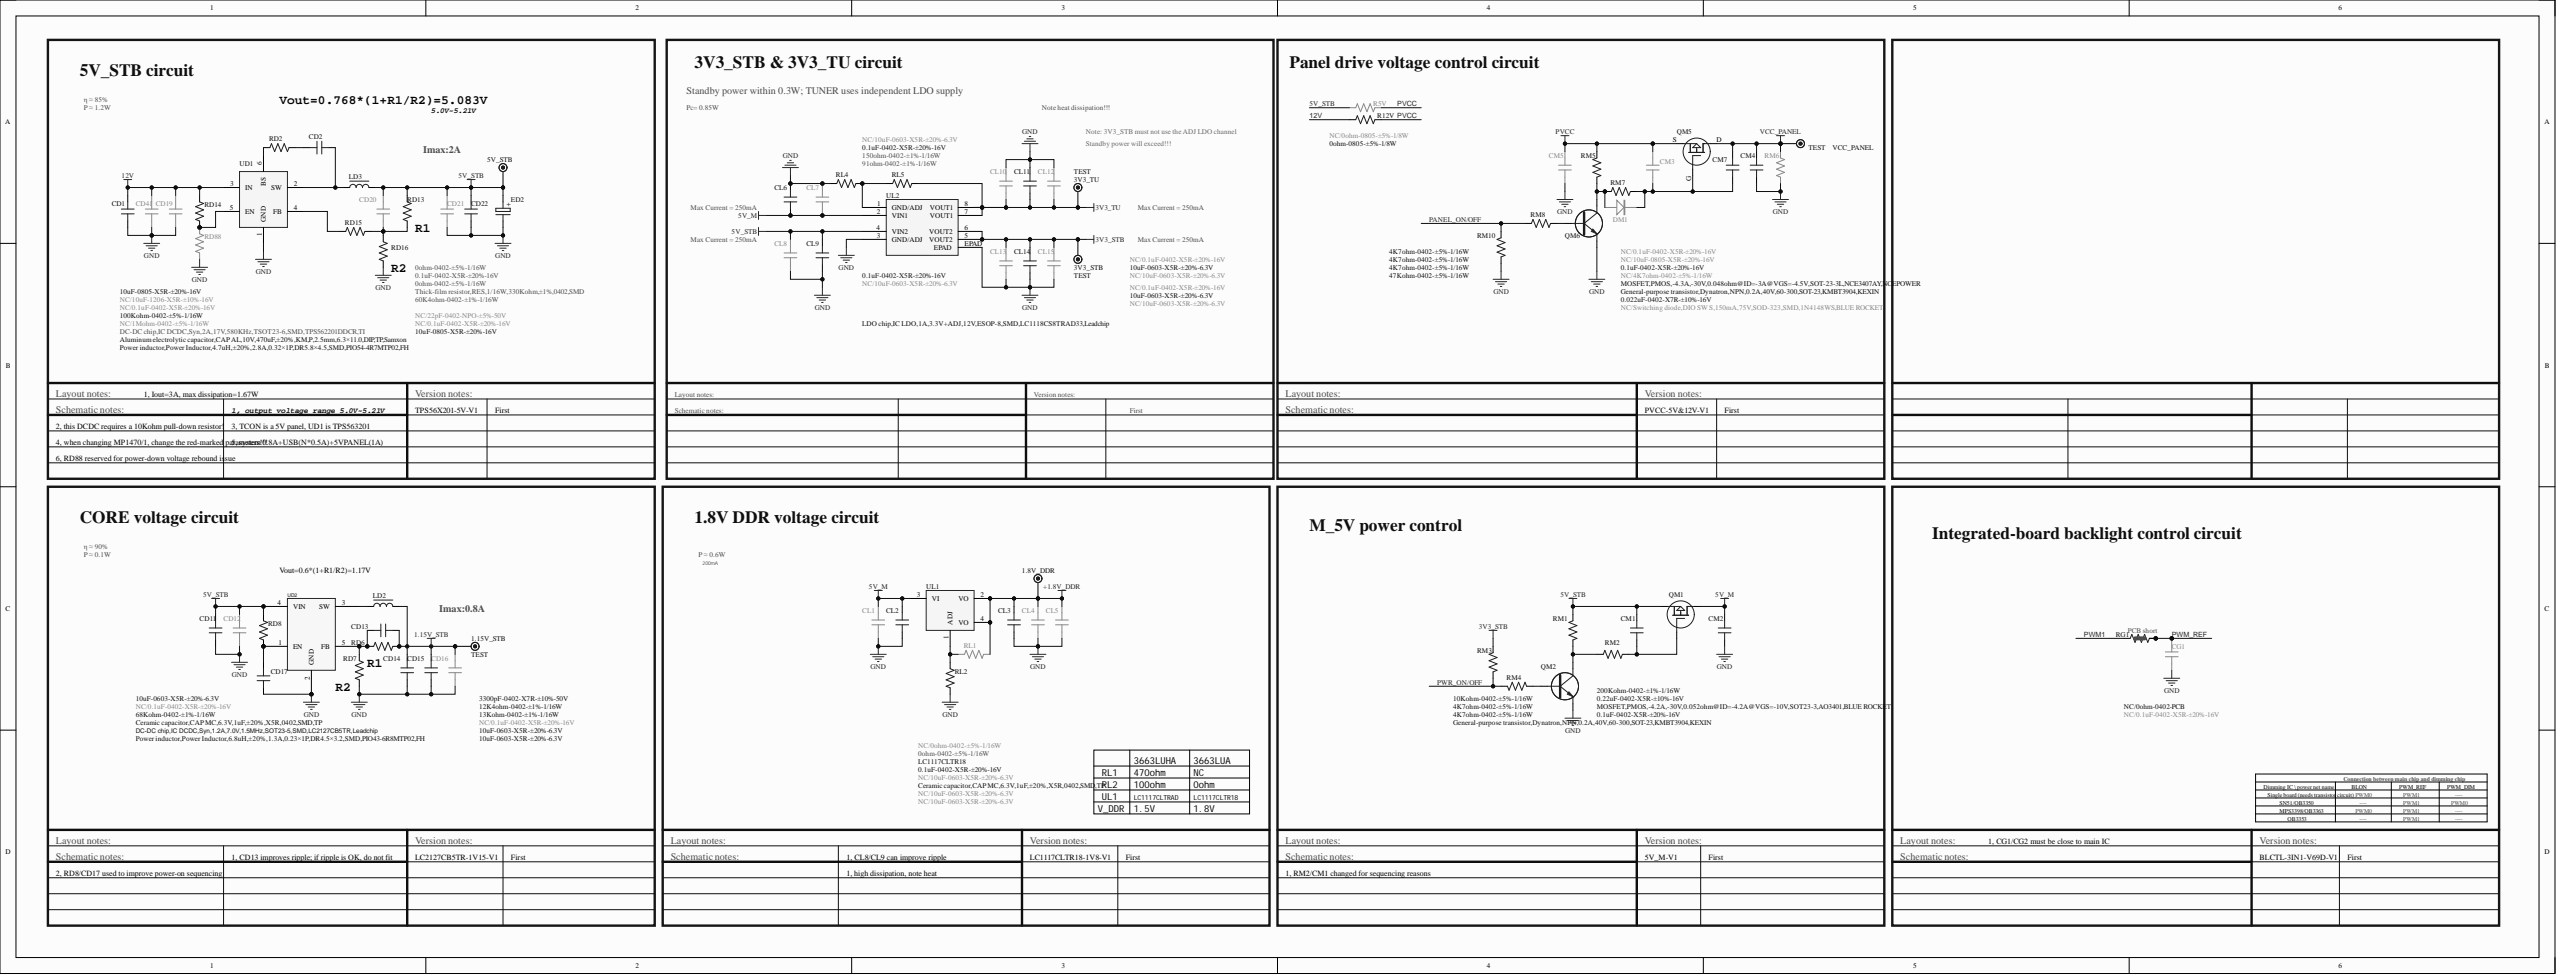Circuit board | Altium Designer | 574 parts | 274 nets | one sheet of the schematic
Parts on this sheet (reference | value | footprint):
1.8V_DDR | TEST | TP
1.15V_STB | TEST | TP
3V3_TU | TEST | TP
CD1 | 10uF-0805-X5R-±20%-16V | C0805
CD2 | 0.1uF-0402-X5R-±20%-16V | C0402
CD11 | 10uF-0603-X5R-±20%-6.3V | C0603
CD12 | NC/0.1uF-0402-X5R-±20%-16V | C0402
CD13 | 3300pF-0402-X7R-±10%-50V | C0402
CD14 | 10uF-0603-X5R-±20%-6.3V | C0603
CD15 | 10uF-0603-X5R-±20%-6.3V | C0603
CD16 | NC/0.1uF-0402-X5R-±20%-16V | C0402
CD17 | Ceramic capacitor,CAP MC,6.3V,1uF,±20%,X5R,0402,SMD,TP | C0402
CD19 | NC/0.1uF-0402-X5R-±20%-16V | C0402
CD20 | NC/22pF-0402-NPO-±5%-50V | C0402
CD21 | NC/0.1uF-0402-X5R-±20%-16V | C0402
CD22 | 10uF-0805-X5R-±20%-16V | C0805
CD41 | NC/10uF-1206-X5R-±10%-16V | C1206
CG1 | NC/0.1uF-0402-X5R-±20%-16V | C0402
CL1 | NC/10uF-0603-X5R-±20%-6.3V | C0603
CL2 | 0.1uF-0402-X5R-±20%-16V | C0402
CL3 | Ceramic capacitor,CAP MC,6.3V,1uF,±20%,X5R,0402,SMD,TP | C0402
CL4 | NC/10uF-0603-X5R-±20%-6.3V | C0603
CL5 | NC/10uF-0603-X5R-±20%-6.3V | C0603
CL6 | 0.1uF-0402-X5R-±20%-16V | C0402
CL7 | NC/10uF-0603-X5R-±20%-6.3V | C0603
CL8 | NC/10uF-0603-X5R-±20%-6.3V | C0603
CL9 | 0.1uF-0402-X5R-±20%-16V | C0402
CL10 | NC/0.1uF-0402-X5R-±20%-16V | C0402
CL11 | 10uF-0603-X5R-±20%-6.3V | C0603
CL12 | NC/10uF-0603-X5R-±20%-6.3V | C0603
CL13 | NC/0.1uF-0402-X5R-±20%-16V | C0402
CL14 | 10uF-0603-X5R-±20%-6.3V | C0603
CL15 | NC/10uF-0603-X5R-±20%-6.3V | C0603
CM1 | 0.22uF-0402-X5R-±10%-16V | C0402
CM2 | 0.1uF-0402-X5R-±20%-16V | C0402
CM3 | NC/0.1uF-0402-X5R-±20%-16V | C0402
CM4 | 0.1uF-0402-X5R-±20%-16V | C0402
CM5 | NC/10uF-0805-X5R-±20%-16V | C0805
CM7 | 0.022uF-0402-X7R-±10%-16V | C0402
DM1 | NC/Switching diode,DIO SW S,150mA,75V,SOD-323,SMD,1N4148WS,BLUE ROCKET | DIODE-S-12
ED2 | Aluminum electrolytic capacitor,CAP AL,10V,470uF,±20%,KM,P,2.5mm,6.3×11.0,DIP,TP,Samxon | EC(6.3*11)-V-2.5
LD2 | Power inductor,Power Inductor,6.8uH,±20%,1.3A,0.23×1P,DR4.5×3.2,SMD,PIO43-6R8MTP02,FH | L(4.5*3.5)-S
LD3 | Power inductor,Power Inductor,4.7uH,±20%,2.8A,0.32×1P,DR5.8×4.5,SMD,PIO54-4R7MTP02,FH | L(6.0*4.5)-S
QM1 | MOSFET,PMOS,-4.2A,-30V,0.052ohm@ID=-4.2A@VGS=-10V,SOT23-3,AO3401,BLUE ROCKET | SOT-23-1
QM2 | General-purpose transistor,Dynatron,NPN,0.2A,40V,60-300,SOT-23,KMBT3904,KEXIN | SOT-23
QM5 | MOSFET,PMOS,-4.3A,-30V,0.048ohm@ID=-3A@VGS=-4.5V,SOT-23-3L,NCE3407AY,NCEPOWER | SOT-23-1
QM6 | General-purpose transistor,Dynatron,NPN,0.2A,40V,60-300,SOT-23,KMBT3904,KEXIN | SOT-23
R5V | NC/0ohm-0805-±5%-1/8W | R0805
R12V | 0ohm-0805-±5%-1/8W | R0805
RD2 | 0ohm-0402-±5%-1/16W | R0402
RD6 | 12K4ohm-0402-±1%-1/16W | R0402
RD7 | 13Kohm-0402-±1%-1/16W | R0402
RD8 | 68Kohm-0402-±1%-1/16W | R0402
RD13 | Thick-film resistor,RES,1/16W,330Kohm,±1%,0402,SMD | R0402
RD14 | 100Kohm-0402-±5%-1/16W | R0402
RD15 | 0ohm-0402-±5%-1/16W | R0402
RD16 | 60K4ohm-0402-±1%-1/16W | R0402
RD88 | NC/1Mohm-0402-±5%-1/16W | R0402
RG1 | NC/0ohm-0402-PCB | R0402SC
RL1 | NC/0ohm-0402-±5%-1/16W | R0402
RL2 | 0ohm-0402-±5%-1/16W | R0402
RL4 | 150ohm-0402-±1%-1/16W | R0402
RL5 | 91ohm-0402-±1%-1/16W | R0402
RM1 | 4K7ohm-0402-±5%-1/16W | R0402
RM2 | 200Kohm-0402-±1%-1/16W | R0402
RM3 | 10Kohm-0402-±5%-1/16W | R0402
RM4 | 4K7ohm-0402-±5%-1/16W | R0402
RM5 | 4K7ohm-0402-±5%-1/16W | R0402
RM6 | NC/4K7ohm-0402-±5%-1/16W | R0402
RM7 | 47Kohm-0402-±5%-1/16W | R0402
RM8 | 4K7ohm-0402-±5%-1/16W | R0402
RM10 | 4K7ohm-0402-±5%-1/16W | R0402
UD1 | DC-DC chip,IC DCDC,Syn,2A,17V,580KHz,TSOT23-6,SMD,TPS562201DDCR,TI | SOT-23-6
UD2 | DC-DC chip,IC DCDC,Syn,1.2A,7.0V,1.5MHz,SOT23-5,SMD,LC2127CB5TR,Leadchip | SOT-23-5
UL1 | LC1117CLTR18 | SOT-223
UL2 | LDO chip,IC LDO,1A,3.3V+ADJ,12V,ESOP-8,SMD,LC1118CS8TRAD33,Leadchip | SOP8/1.27-3
Nets of these parts (net: part-pin ...):
VCC_PANEL: CM4-1 CM7-2 QM5-D RM6-1
PWR_ON/OFF: RM3-2 RM4-2
PWM_REF: CG1-1 RG1-2 RG1-3
PWM1: RG1-1
PVCC: CM3-2 CM5-2 QM5-S R5V-2 R12V-2 RM5-2
PANEL_ON/OFF: RM8-1 RM10-1
NetRL4_2: RL4-2 RL5-1 UL2-1
NetRL1_2: RL1-2 RL2-1 UL1-1
NetRD15_1: RD15-1 UD1-4
NetRD14_2: RD14-2 RD88-2 UD1-5
NetRD2_1: RD2-1 UD1-6
NetQM6_B: QM6-B RM8-2
NetQM2_C: QM2-C RM1-1 RM2-1
NetQM2_B: QM2-B RM4-1
NetLD2_1: LD2-1 UD2-3
NetDM1_A: DM1-A QM6-C RM5-1 RM7-1
NetCM3_1: CM3-1 CM7-1 DM1-K QM5-G RM7-2
NetCM1_2: CM1-2 QM1-G RM2-2
NetCD20_2: CD20-2 RD13-1 RD15-2 RD16-2
NetCD17_2: CD17-2 RD8-2 UD2-1
NetCD13_2: CD13-2 RD6-1 RD7-2 UD2-5
NetCD2_2: CD2-2 LD3-1 UD1-2
NetCD2_1: CD2-1 RD2-2
GND: CD1-2 CD11-1 CD12-2 CD14-1 CD15-1 CD16-1 CD17-1 CD19-2 CD21-2 CD22-2 CD41-1 CG1-2 CL1-1 CL2-1 CL3-1 CL4-1 CL5-1 CL6-1 CL7-1 CL8-1 CL9-1 CL10-1 CL11-2 CL12-2 CL13-2 CL14-2 CL15-1 CM2-2 CM4-2 CM5-1 ED2-2 QM2-E QM6-E RD7-1 RD16-1 RD88-1 RL2-2 RL4-1 RM6-2 RM10-2 UD1-1 UD2-2 UL2-3 UL2-EPAD
+1.8V_DDR: 1.8V_DDR-1 CL3-2 CL4-2 CL5-2 RL1-1 UL1-2 UL1-4
12V: CD1-1 CD19-1 CD41-2 R12V-1 RD14-1 UD1-3
5V_STB: CD11-2 CD12-1 CD20-1 CD21-1 CD22-1 CL8-2 CL9-2 CM1-1 ED2-1 LD3-2 QM1-S R5V-1 RD8-1 RD13-2 RM1-2 UD2-4 UL2-4
5V_M: CL1-2 CL2-2 CL6-2 CL7-2 CM2-1 QM1-D UL1-3 UL2-2
3V3_TU: 3V3_TU-1 CL10-2 CL11-1 CL12-1 RL5-2 UL2-7 UL2-8
3V3_STB: CL13-1 CL14-1 CL15-2 RM3-1 UL2-5 UL2-6
1.15V_STB: 1.15V_STB-1 CD13-1 CD14-2 CD15-2 CD16-2 LD2-2 RD6-2